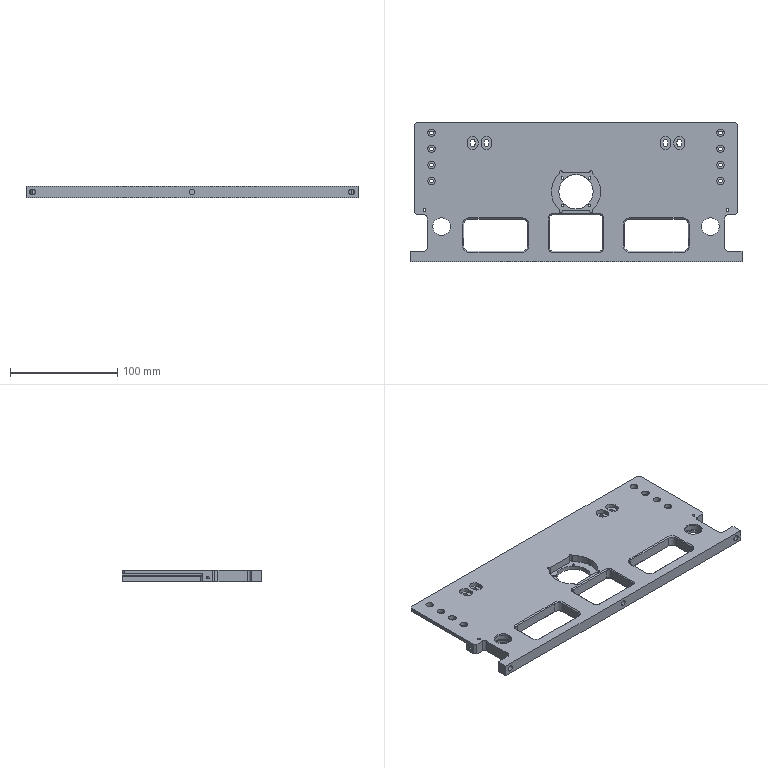Part | NX | features BREP 1 | 1 solid | 491 faces | box 310 x 130.5 x 11 mm | volume 241752 mm3 | plane 234 | cylinder 177 | cone 80 | commonest cylinder face diameters 6 x44 10 x32 2.5 x16 3.4 x16 7 x16 3 x12